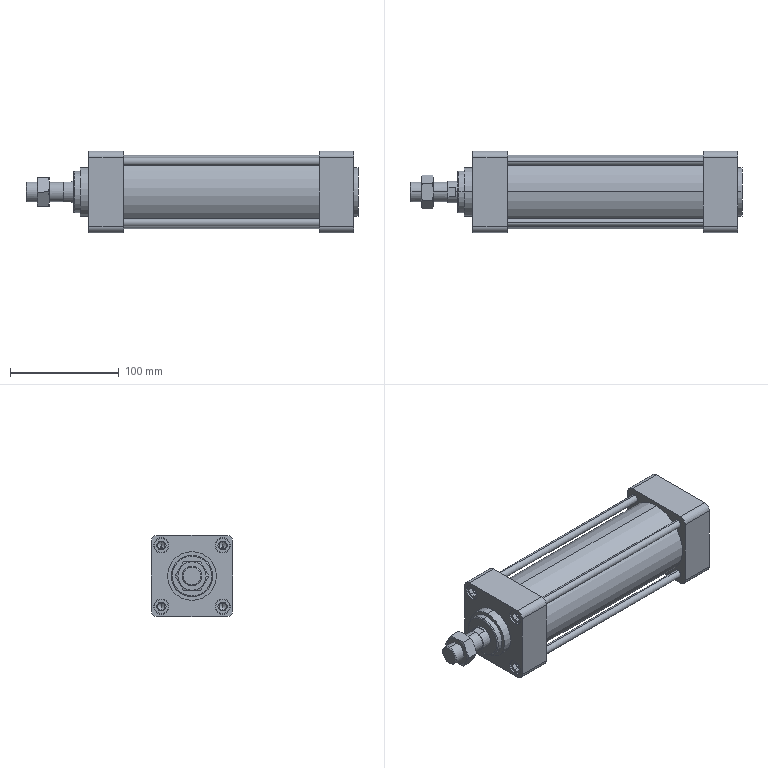Part | SolidWorks | 3 solids | 264 faces | box 306 x 75 x 75 mm | volume 647112 mm3 | plane 128 | cylinder 92 | cone 42 | spline 2 | commonest cylinder face diameters 6.647 x16 13 x16 14 x16 7.2 x8 12 x8 9.8 x4